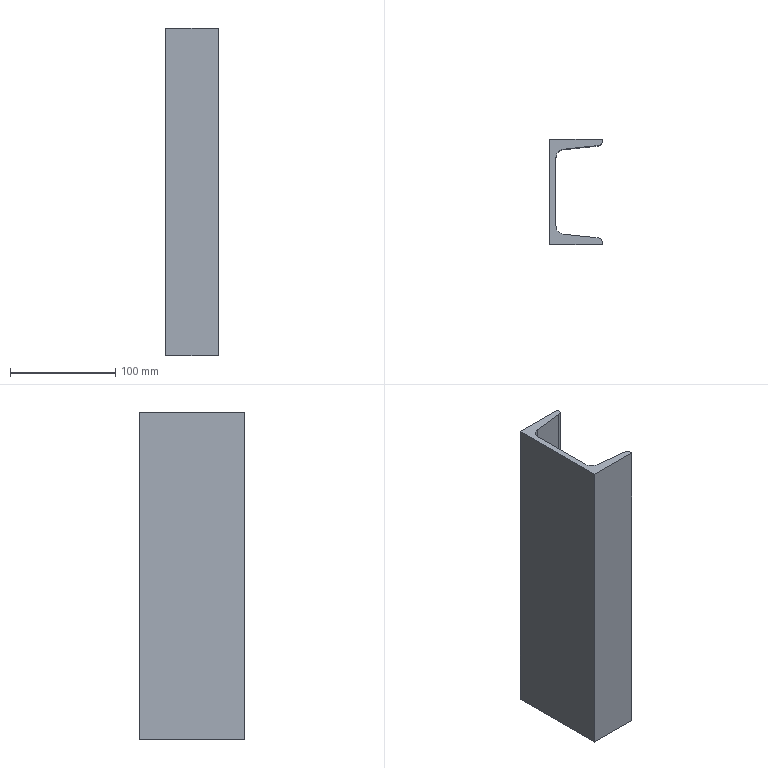Part | STEP file | ISO 657_11 CH 100 x 10 1784900456176 | 1 solid | 14 faces | box 50 x 100 x 312 mm | volume 408796 mm3 | plane 10 | cylinder 4 | commonest cylinder face diameters 9 x2 16 x2
STEP:
#1=CARTESIAN_POINT('',(4.39,-32.479,362.));
#2=VERTEX_POINT('',#1);
#3=CARTESIAN_POINT('',(11.554,-40.435,362.));
#4=VERTEX_POINT('',#3);
#5=CARTESIAN_POINT('',(12.39,-32.479,362.));
#6=DIRECTION('',(0.,0.,1.));
#7=DIRECTION('',(-1.,0.,0.));
#8=AXIS2_PLACEMENT_3D('',#5,#6,#7);
#9=CIRCLE('',#8,8.);
#10=EDGE_CURVE('',#2,#4,#9,.T.);
#11=ORIENTED_EDGE('',*,*,#10,.T.);
#12=CARTESIAN_POINT('',(11.554,-40.435,50.));
#13=VERTEX_POINT('',#12);
#14=CARTESIAN_POINT('',(11.554,-40.435,0.));
#15=DIRECTION('',(0.,0.,1.));
#16=VECTOR('',#15,10.);
#17=LINE('',#14,#16);
#18=EDGE_CURVE('',#13,#4,#17,.T.);
#19=ORIENTED_EDGE('',*,*,#18,.F.);
#20=CARTESIAN_POINT('',(4.39,-32.479,50.));
#21=VERTEX_POINT('',#20);
#22=CARTESIAN_POINT('',(12.39,-32.479,50.));
#23=DIRECTION('',(0.,0.,1.));
#24=DIRECTION('',(-1.,0.,0.));
#25=AXIS2_PLACEMENT_3D('',#22,#23,#24);
#26=CIRCLE('',#25,8.);
#27=EDGE_CURVE('',#21,#13,#26,.T.);
#28=ORIENTED_EDGE('',*,*,#27,.F.);
#29=CARTESIAN_POINT('',(4.39,-32.479,0.));
#30=DIRECTION('',(0.,0.,1.));
#31=VECTOR('',#30,10.);
#32=LINE('',#29,#31);
#33=EDGE_CURVE('',#21,#2,#32,.T.);
#34=ORIENTED_EDGE('',*,*,#33,.T.);
#35=EDGE_LOOP('',(#11,#19,#28,#34));
#36=FACE_OUTER_BOUND('',#35,.T.);
#37=CARTESIAN_POINT('',(12.39,-32.479,0.));
#38=DIRECTION('',(0.,0.,1.));
#39=DIRECTION('',(-1.,0.,0.));
#40=AXIS2_PLACEMENT_3D('',#37,#38,#39);
#41=CYLINDRICAL_SURFACE('',#40,8.);
#42=ADVANCED_FACE('',(#36),#41,.F.);
#43=CARTESIAN_POINT('',(44.46,-43.894,362.));
#44=VERTEX_POINT('',#43);
#45=CARTESIAN_POINT('',(15.355,-40.835,362.));
#46=DIRECTION('',(0.9945,-0.1045,0.));
#47=VECTOR('',#46,10.);
#48=LINE('',#45,#47);
#49=EDGE_CURVE('',#4,#44,#48,.T.);
#50=ORIENTED_EDGE('',*,*,#49,.T.);
#51=CARTESIAN_POINT('',(44.46,-43.894,50.));
#52=VERTEX_POINT('',#51);
#53=CARTESIAN_POINT('',(44.46,-43.894,0.));
#54=DIRECTION('',(0.,0.,1.));
#55=VECTOR('',#54,10.);
#56=LINE('',#53,#55);
#57=EDGE_CURVE('',#52,#44,#56,.T.);
#58=ORIENTED_EDGE('',*,*,#57,.F.);
#59=CARTESIAN_POINT('',(15.355,-40.835,50.));
#60=DIRECTION('',(0.9945,-0.1045,0.));
#61=VECTOR('',#60,10.);
#62=LINE('',#59,#61);
#63=EDGE_CURVE('',#13,#52,#62,.T.);
#64=ORIENTED_EDGE('',*,*,#63,.F.);
#65=ORIENTED_EDGE('',*,*,#18,.T.);
#66=EDGE_LOOP('',(#50,#58,#64,#65));
#67=FACE_OUTER_BOUND('',#66,.T.);
#68=CARTESIAN_POINT('',(11.554,-40.435,0.));
#69=DIRECTION('',(0.1045,0.9945,0.));
#70=DIRECTION('',(0.,0.,1.));
#71=AXIS2_PLACEMENT_3D('',#68,#69,#70);
#72=PLANE('',#71);
#73=ADVANCED_FACE('',(#67),#72,.T.);
#74=CARTESIAN_POINT('',(48.49,-48.369,362.));
#75=VERTEX_POINT('',#74);
#76=CARTESIAN_POINT('',(43.99,-48.369,362.));
#77=DIRECTION('',(0.,0.,-1.));
#78=DIRECTION('',(-1.,0.,0.));
#79=AXIS2_PLACEMENT_3D('',#76,#77,#78);
#80=CIRCLE('',#79,4.5);
#81=EDGE_CURVE('',#44,#75,#80,.T.);
#82=ORIENTED_EDGE('',*,*,#81,.T.);
#83=CARTESIAN_POINT('',(48.49,-48.369,50.));
#84=VERTEX_POINT('',#83);
#85=CARTESIAN_POINT('',(48.49,-48.369,0.));
#86=DIRECTION('',(0.,0.,1.));
#87=VECTOR('',#86,10.);
#88=LINE('',#85,#87);
#89=EDGE_CURVE('',#84,#75,#88,.T.);
#90=ORIENTED_EDGE('',*,*,#89,.F.);
#91=CARTESIAN_POINT('',(43.99,-48.369,50.));
#92=DIRECTION('',(0.,0.,-1.));
#93=DIRECTION('',(-1.,0.,0.));
#94=AXIS2_PLACEMENT_3D('',#91,#92,#93);
#95=CIRCLE('',#94,4.5);
#96=EDGE_CURVE('',#52,#84,#95,.T.);
#97=ORIENTED_EDGE('',*,*,#96,.F.);
#98=ORIENTED_EDGE('',*,*,#57,.T.);
#99=EDGE_LOOP('',(#82,#90,#97,#98));
#100=FACE_OUTER_BOUND('',#99,.T.);
#101=CARTESIAN_POINT('',(43.99,-48.369,0.));
#102=DIRECTION('',(0.,0.,1.));
#103=DIRECTION('',(-1.,0.,0.));
#104=AXIS2_PLACEMENT_3D('',#101,#102,#103);
#105=CYLINDRICAL_SURFACE('',#104,4.5);
#106=ADVANCED_FACE('',(#100),#105,.T.);
#107=CARTESIAN_POINT('',(48.49,-50.,362.));
#108=VERTEX_POINT('',#107);
#109=CARTESIAN_POINT('',(48.49,-24.185,362.));
#110=DIRECTION('',(0.,-1.,0.));
#111=VECTOR('',#110,10.);
#112=LINE('',#109,#111);
#113=EDGE_CURVE('',#75,#108,#112,.T.);
#114=ORIENTED_EDGE('',*,*,#113,.T.);
#115=CARTESIAN_POINT('',(48.49,-50.,50.));
#116=VERTEX_POINT('',#115);
#117=CARTESIAN_POINT('',(48.49,-50.,0.));
#118=DIRECTION('',(0.,0.,1.));
#119=VECTOR('',#118,10.);
#120=LINE('',#117,#119);
#121=EDGE_CURVE('',#116,#108,#120,.T.);
#122=ORIENTED_EDGE('',*,*,#121,.F.);
#123=CARTESIAN_POINT('',(48.49,-24.185,50.));
#124=DIRECTION('',(0.,-1.,0.));
#125=VECTOR('',#124,10.);
#126=LINE('',#123,#125);
#127=EDGE_CURVE('',#84,#116,#126,.T.);
#128=ORIENTED_EDGE('',*,*,#127,.F.);
#129=ORIENTED_EDGE('',*,*,#89,.T.);
#130=EDGE_LOOP('',(#114,#122,#128,#129));
#131=FACE_OUTER_BOUND('',#130,.T.);
#132=CARTESIAN_POINT('',(48.49,-48.369,0.));
#133=DIRECTION('',(1.,0.,0.));
#134=DIRECTION('',(0.,0.,-1.));
#135=AXIS2_PLACEMENT_3D('',#132,#133,#134);
#136=PLANE('',#135);
#137=ADVANCED_FACE('',(#131),#136,.T.);
#138=CARTESIAN_POINT('',(-1.51,-50.,362.));
#139=VERTEX_POINT('',#138);
#140=CARTESIAN_POINT('',(35.99,-50.,362.));
#141=DIRECTION('',(-1.,0.,0.));
#142=VECTOR('',#141,10.);
#143=LINE('',#140,#142);
#144=EDGE_CURVE('',#108,#139,#143,.T.);
#145=ORIENTED_EDGE('',*,*,#144,.T.);
#146=CARTESIAN_POINT('',(-1.51,-50.,50.));
#147=VERTEX_POINT('',#146);
#148=CARTESIAN_POINT('',(-1.51,-50.,0.));
#149=DIRECTION('',(0.,0.,1.));
#150=VECTOR('',#149,10.);
#151=LINE('',#148,#150);
#152=EDGE_CURVE('',#147,#139,#151,.T.);
#153=ORIENTED_EDGE('',*,*,#152,.F.);
#154=CARTESIAN_POINT('',(35.99,-50.,50.));
#155=DIRECTION('',(-1.,0.,0.));
#156=VECTOR('',#155,10.);
#157=LINE('',#154,#156);
#158=EDGE_CURVE('',#116,#147,#157,.T.);
#159=ORIENTED_EDGE('',*,*,#158,.F.);
#160=ORIENTED_EDGE('',*,*,#121,.T.);
#161=EDGE_LOOP('',(#145,#153,#159,#160));
#162=FACE_OUTER_BOUND('',#161,.T.);
#163=CARTESIAN_POINT('',(48.49,-50.,0.));
#164=DIRECTION('',(0.,-1.,0.));
#165=DIRECTION('',(0.,0.,-1.));
#166=AXIS2_PLACEMENT_3D('',#163,#164,#165);
#167=PLANE('',#166);
#168=ADVANCED_FACE('',(#162),#167,.T.);
#169=CARTESIAN_POINT('',(-1.51,50.,362.));
#170=VERTEX_POINT('',#169);
#171=CARTESIAN_POINT('',(-1.51,0.,362.));
#172=DIRECTION('',(0.,1.,0.));
#173=VECTOR('',#172,10.);
#174=LINE('',#171,#173);
#175=EDGE_CURVE('',#139,#170,#174,.T.);
#176=ORIENTED_EDGE('',*,*,#175,.T.);
#177=CARTESIAN_POINT('',(-1.51,50.,50.));
#178=VERTEX_POINT('',#177);
#179=CARTESIAN_POINT('',(-1.51,50.,0.));
#180=DIRECTION('',(0.,0.,1.));
#181=VECTOR('',#180,10.);
#182=LINE('',#179,#181);
#183=EDGE_CURVE('',#178,#170,#182,.T.);
#184=ORIENTED_EDGE('',*,*,#183,.F.);
#185=CARTESIAN_POINT('',(-1.51,0.,50.));
#186=DIRECTION('',(0.,1.,0.));
#187=VECTOR('',#186,10.);
#188=LINE('',#185,#187);
#189=EDGE_CURVE('',#147,#178,#188,.T.);
#190=ORIENTED_EDGE('',*,*,#189,.F.);
#191=ORIENTED_EDGE('',*,*,#152,.T.);
#192=EDGE_LOOP('',(#176,#184,#190,#191));
#193=FACE_OUTER_BOUND('',#192,.T.);
#194=CARTESIAN_POINT('',(-1.51,0.,0.));
#195=DIRECTION('',(-1.,0.,0.));
#196=DIRECTION('',(0.,0.,1.));
#197=AXIS2_PLACEMENT_3D('',#194,#195,#196);
#198=PLANE('',#197);
#199=ADVANCED_FACE('',(#193),#198,.T.);
#200=CARTESIAN_POINT('',(48.49,50.,362.));
#201=VERTEX_POINT('',#200);
#202=CARTESIAN_POINT('',(10.99,50.,362.));
#203=DIRECTION('',(1.,0.,0.));
#204=VECTOR('',#203,10.);
#205=LINE('',#202,#204);
#206=EDGE_CURVE('',#170,#201,#205,.T.);
#207=ORIENTED_EDGE('',*,*,#206,.T.);
#208=CARTESIAN_POINT('',(48.49,50.,50.));
#209=VERTEX_POINT('',#208);
#210=CARTESIAN_POINT('',(48.49,50.,0.));
#211=DIRECTION('',(0.,0.,1.));
#212=VECTOR('',#211,10.);
#213=LINE('',#210,#212);
#214=EDGE_CURVE('',#209,#201,#213,.T.);
#215=ORIENTED_EDGE('',*,*,#214,.F.);
#216=CARTESIAN_POINT('',(10.99,50.,50.));
#217=DIRECTION('',(1.,0.,0.));
#218=VECTOR('',#217,10.);
#219=LINE('',#216,#218);
#220=EDGE_CURVE('',#178,#209,#219,.T.);
#221=ORIENTED_EDGE('',*,*,#220,.F.);
#222=ORIENTED_EDGE('',*,*,#183,.T.);
#223=EDGE_LOOP('',(#207,#215,#221,#222));
#224=FACE_OUTER_BOUND('',#223,.T.);
#225=CARTESIAN_POINT('',(-1.51,50.,0.));
#226=DIRECTION('',(0.,1.,0.));
#227=DIRECTION('',(0.,0.,1.));
#228=AXIS2_PLACEMENT_3D('',#225,#226,#227);
#229=PLANE('',#228);
#230=ADVANCED_FACE('',(#224),#229,.T.);
#231=CARTESIAN_POINT('',(48.49,48.369,362.));
#232=VERTEX_POINT('',#231);
#233=CARTESIAN_POINT('',(48.49,25.,362.));
#234=DIRECTION('',(0.,-1.,0.));
#235=VECTOR('',#234,10.);
#236=LINE('',#233,#235);
#237=EDGE_CURVE('',#201,#232,#236,.T.);
#238=ORIENTED_EDGE('',*,*,#237,.T.);
#239=CARTESIAN_POINT('',(48.49,48.369,50.));
#240=VERTEX_POINT('',#239);
#241=CARTESIAN_POINT('',(48.49,48.369,0.));
#242=DIRECTION('',(0.,0.,1.));
#243=VECTOR('',#242,10.);
#244=LINE('',#241,#243);
#245=EDGE_CURVE('',#240,#232,#244,.T.);
#246=ORIENTED_EDGE('',*,*,#245,.F.);
#247=CARTESIAN_POINT('',(48.49,25.,50.));
#248=DIRECTION('',(0.,-1.,0.));
#249=VECTOR('',#248,10.);
#250=LINE('',#247,#249);
#251=EDGE_CURVE('',#209,#240,#250,.T.);
#252=ORIENTED_EDGE('',*,*,#251,.F.);
#253=ORIENTED_EDGE('',*,*,#214,.T.);
#254=EDGE_LOOP('',(#238,#246,#252,#253));
#255=FACE_OUTER_BOUND('',#254,.T.);
#256=CARTESIAN_POINT('',(48.49,50.,0.));
#257=DIRECTION('',(1.,0.,0.));
#258=DIRECTION('',(0.,0.,-1.));
#259=AXIS2_PLACEMENT_3D('',#256,#257,#258);
#260=PLANE('',#259);
#261=ADVANCED_FACE('',(#255),#260,.T.);
#262=CARTESIAN_POINT('',(44.46,43.894,362.));
#263=VERTEX_POINT('',#262);
#264=CARTESIAN_POINT('',(43.99,48.369,362.));
#265=DIRECTION('',(0.,0.,-1.));
#266=DIRECTION('',(-0.1045,0.9945,0.));
#267=AXIS2_PLACEMENT_3D('',#264,#265,#266);
#268=CIRCLE('',#267,4.5);
#269=EDGE_CURVE('',#232,#263,#268,.T.);
#270=ORIENTED_EDGE('',*,*,#269,.T.);
#271=CARTESIAN_POINT('',(44.46,43.894,50.));
#272=VERTEX_POINT('',#271);
#273=CARTESIAN_POINT('',(44.46,43.894,0.));
#274=DIRECTION('',(0.,0.,1.));
#275=VECTOR('',#274,10.);
#276=LINE('',#273,#275);
#277=EDGE_CURVE('',#272,#263,#276,.T.);
#278=ORIENTED_EDGE('',*,*,#277,.F.);
#279=CARTESIAN_POINT('',(43.99,48.369,50.));
#280=DIRECTION('',(0.,0.,-1.));
#281=DIRECTION('',(-0.1045,0.9945,0.));
#282=AXIS2_PLACEMENT_3D('',#279,#280,#281);
#283=CIRCLE('',#282,4.5);
#284=EDGE_CURVE('',#240,#272,#283,.T.);
#285=ORIENTED_EDGE('',*,*,#284,.F.);
#286=ORIENTED_EDGE('',*,*,#245,.T.);
#287=EDGE_LOOP('',(#270,#278,#285,#286));
#288=FACE_OUTER_BOUND('',#287,.T.);
#289=CARTESIAN_POINT('',(43.99,48.369,0.));
#290=DIRECTION('',(0.,0.,1.));
#291=DIRECTION('',(-0.1045,0.9945,0.));
#292=AXIS2_PLACEMENT_3D('',#289,#290,#291);
#293=CYLINDRICAL_SURFACE('',#292,4.5);
#294=ADVANCED_FACE('',(#288),#293,.T.);
#295=CARTESIAN_POINT('',(11.554,40.435,362.));
#296=VERTEX_POINT('',#295);
#297=CARTESIAN_POINT('',(31.808,42.564,362.));
#298=DIRECTION('',(-0.9945,-0.1045,0.));
#299=VECTOR('',#298,10.);
#300=LINE('',#297,#299);
#301=EDGE_CURVE('',#263,#296,#300,.T.);
#302=ORIENTED_EDGE('',*,*,#301,.T.);
#303=CARTESIAN_POINT('',(11.554,40.435,50.));
#304=VERTEX_POINT('',#303);
#305=CARTESIAN_POINT('',(11.554,40.435,0.));
#306=DIRECTION('',(0.,0.,1.));
#307=VECTOR('',#306,10.);
#308=LINE('',#305,#307);
#309=EDGE_CURVE('',#304,#296,#308,.T.);
#310=ORIENTED_EDGE('',*,*,#309,.F.);
#311=CARTESIAN_POINT('',(31.808,42.564,50.));
#312=DIRECTION('',(-0.9945,-0.1045,0.));
#313=VECTOR('',#312,10.);
#314=LINE('',#311,#313);
#315=EDGE_CURVE('',#272,#304,#314,.T.);
#316=ORIENTED_EDGE('',*,*,#315,.F.);
#317=ORIENTED_EDGE('',*,*,#277,.T.);
#318=EDGE_LOOP('',(#302,#310,#316,#317));
#319=FACE_OUTER_BOUND('',#318,.T.);
#320=CARTESIAN_POINT('',(44.46,43.894,0.));
#321=DIRECTION('',(0.1045,-0.9945,0.));
#322=DIRECTION('',(0.,0.,-1.));
#323=AXIS2_PLACEMENT_3D('',#320,#321,#322);
#324=PLANE('',#323);
#325=ADVANCED_FACE('',(#319),#324,.T.);
#326=CARTESIAN_POINT('',(4.39,32.479,362.));
#327=VERTEX_POINT('',#326);
#328=CARTESIAN_POINT('',(12.39,32.479,362.));
#329=DIRECTION('',(0.,0.,1.));
#330=DIRECTION('',(-0.1045,0.9945,0.));
#331=AXIS2_PLACEMENT_3D('',#328,#329,#330);
#332=CIRCLE('',#331,8.);
#333=EDGE_CURVE('',#296,#327,#332,.T.);
#334=ORIENTED_EDGE('',*,*,#333,.T.);
#335=CARTESIAN_POINT('',(4.39,32.479,50.));
#336=VERTEX_POINT('',#335);
#337=CARTESIAN_POINT('',(4.39,32.479,0.));
#338=DIRECTION('',(0.,0.,1.));
#339=VECTOR('',#338,10.);
#340=LINE('',#337,#339);
#341=EDGE_CURVE('',#336,#327,#340,.T.);
#342=ORIENTED_EDGE('',*,*,#341,.F.);
#343=CARTESIAN_POINT('',(12.39,32.479,50.));
#344=DIRECTION('',(0.,0.,1.));
#345=DIRECTION('',(-0.1045,0.9945,0.));
#346=AXIS2_PLACEMENT_3D('',#343,#344,#345);
#347=CIRCLE('',#346,8.);
#348=EDGE_CURVE('',#304,#336,#347,.T.);
#349=ORIENTED_EDGE('',*,*,#348,.F.);
#350=ORIENTED_EDGE('',*,*,#309,.T.);
#351=EDGE_LOOP('',(#334,#342,#349,#350));
#352=FACE_OUTER_BOUND('',#351,.T.);
#353=CARTESIAN_POINT('',(12.39,32.479,0.));
#354=DIRECTION('',(0.,0.,1.));
#355=DIRECTION('',(-0.1045,0.9945,0.));
#356=AXIS2_PLACEMENT_3D('',#353,#354,#355);
#357=CYLINDRICAL_SURFACE('',#356,8.);
#358=ADVANCED_FACE('',(#352),#357,.F.);
#359=CARTESIAN_POINT('',(4.39,0.,362.));
#360=DIRECTION('',(0.,-1.,0.));
#361=VECTOR('',#360,10.);
#362=LINE('',#359,#361);
#363=EDGE_CURVE('',#327,#2,#362,.T.);
#364=ORIENTED_EDGE('',*,*,#363,.T.);
#365=ORIENTED_EDGE('',*,*,#33,.F.);
#366=CARTESIAN_POINT('',(4.39,0.,50.));
#367=DIRECTION('',(0.,-1.,0.));
#368=VECTOR('',#367,10.);
#369=LINE('',#366,#368);
#370=EDGE_CURVE('',#336,#21,#369,.T.);
#371=ORIENTED_EDGE('',*,*,#370,.F.);
#372=ORIENTED_EDGE('',*,*,#341,.T.);
#373=EDGE_LOOP('',(#364,#365,#371,#372));
#374=FACE_OUTER_BOUND('',#373,.T.);
#375=CARTESIAN_POINT('',(4.39,0.,0.));
#376=DIRECTION('',(1.,0.,0.));
#377=DIRECTION('',(0.,0.,-1.));
#378=AXIS2_PLACEMENT_3D('',#375,#376,#377);
#379=PLANE('',#378);
#380=ADVANCED_FACE('',(#374),#379,.T.);
#381=ORIENTED_EDGE('',*,*,#220,.T.);
#382=ORIENTED_EDGE('',*,*,#251,.T.);
#383=ORIENTED_EDGE('',*,*,#284,.T.);
#384=ORIENTED_EDGE('',*,*,#315,.T.);
#385=ORIENTED_EDGE('',*,*,#348,.T.);
#386=ORIENTED_EDGE('',*,*,#370,.T.);
#387=ORIENTED_EDGE('',*,*,#27,.T.);
#388=ORIENTED_EDGE('',*,*,#63,.T.);
#389=ORIENTED_EDGE('',*,*,#96,.T.);
#390=ORIENTED_EDGE('',*,*,#127,.T.);
#391=ORIENTED_EDGE('',*,*,#158,.T.);
#392=ORIENTED_EDGE('',*,*,#189,.T.);
#393=EDGE_LOOP('',(#381,#382,#383,#384,#385,#386,#387,#388,#389,#390,#391,#392));
#394=FACE_OUTER_BOUND('',#393,.T.);
#395=CARTESIAN_POINT('',(23.49,0.,50.));
#396=DIRECTION('',(0.,0.,1.));
#397=DIRECTION('',(1.,0.,0.));
#398=AXIS2_PLACEMENT_3D('',#395,#396,#397);
#399=PLANE('',#398);
#400=ADVANCED_FACE('',(#394),#399,.F.);
#401=ORIENTED_EDGE('',*,*,#206,.F.);
#402=ORIENTED_EDGE('',*,*,#175,.F.);
#403=ORIENTED_EDGE('',*,*,#144,.F.);
#404=ORIENTED_EDGE('',*,*,#113,.F.);
#405=ORIENTED_EDGE('',*,*,#81,.F.);
#406=ORIENTED_EDGE('',*,*,#49,.F.);
#407=ORIENTED_EDGE('',*,*,#10,.F.);
#408=ORIENTED_EDGE('',*,*,#363,.F.);
#409=ORIENTED_EDGE('',*,*,#333,.F.);
#410=ORIENTED_EDGE('',*,*,#301,.F.);
#411=ORIENTED_EDGE('',*,*,#269,.F.);
#412=ORIENTED_EDGE('',*,*,#237,.F.);
#413=EDGE_LOOP('',(#401,#402,#403,#404,#405,#406,#407,#408,#409,#410,#411,#412));
#414=FACE_OUTER_BOUND('',#413,.T.);
#415=CARTESIAN_POINT('',(23.49,0.,362.));
#416=DIRECTION('',(0.,0.,1.));
#417=DIRECTION('',(1.,0.,0.));
#418=AXIS2_PLACEMENT_3D('',#415,#416,#417);
#419=PLANE('',#418);
#420=ADVANCED_FACE('',(#414),#419,.T.);
#421=CLOSED_SHELL('',(#42,#73,#106,#137,#168,#199,#230,#261,#294,#325,#358,#380,#400,#420));
#422=MANIFOLD_SOLID_BREP('',#421);
#423=(LENGTH_UNIT()NAMED_UNIT(*)SI_UNIT(.MILLI.,.METRE.));
#424=UNCERTAINTY_MEASURE_WITH_UNIT(LENGTH_MEASURE(0.01),#423,'','');
#425=(NAMED_UNIT(*)PLANE_ANGLE_UNIT()SI_UNIT($,.RADIAN.));
#426=(NAMED_UNIT(*)SI_UNIT($,.STERADIAN.)SOLID_ANGLE_UNIT());
#427=(GEOMETRIC_REPRESENTATION_CONTEXT(3)GLOBAL_UNCERTAINTY_ASSIGNED_CONTEXT((#424))GLOBAL_UNIT_ASSIGNED_CONTEXT((#423,#425,#426))REPRESENTATION_CONTEXT('',''));
#428=ADVANCED_BREP_SHAPE_REPRESENTATION('',(#422),#427);